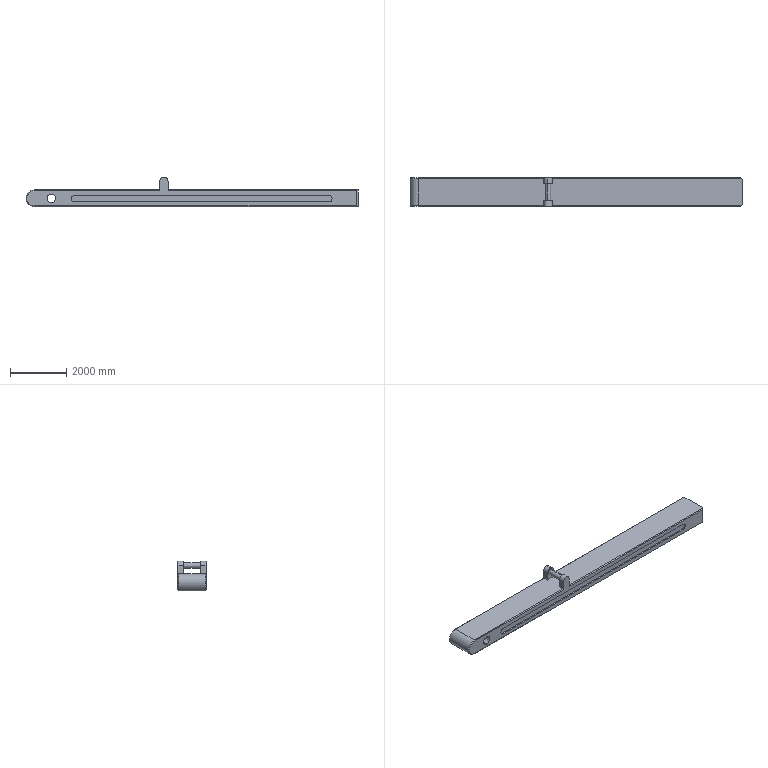Part | SolidWorks | features ICE 4, Chamfer 2, MirrorPattern 2, Extrusion 1 | 1 solid | 44 faces | box 11800 x 1000 x 1050 mm | volume 3596750717 mm3 | plane 30 | cylinder 12 | cone 2 | commonest cylinder face diameters 300 x5 238.236 x4 200 x2 600 x1
STEP:
#1=CARTESIAN_POINT('',(4600.,200.,400.));
#2=VERTEX_POINT('',#1);
#3=CARTESIAN_POINT('',(4600.,200.,200.));
#4=VERTEX_POINT('',#3);
#5=CARTESIAN_POINT('',(4600.,200.,300.));
#6=DIRECTION('',(0.,1.,0.));
#7=DIRECTION('',(0.,0.,-1.));
#8=AXIS2_PLACEMENT_3D('',#5,#6,#7);
#9=CIRCLE('',#8,100.);
#10=EDGE_CURVE('',#2,#4,#9,.T.);
#11=ORIENTED_EDGE('',*,*,#10,.T.);
#12=CARTESIAN_POINT('',(4600.,800.,200.));
#13=VERTEX_POINT('',#12);
#14=CARTESIAN_POINT('',(4600.,100.,200.));
#15=DIRECTION('',(0.,1.,0.));
#16=VECTOR('',#15,1000.);
#17=LINE('',#14,#16);
#18=EDGE_CURVE('',#4,#13,#17,.T.);
#19=ORIENTED_EDGE('',*,*,#18,.T.);
#20=CARTESIAN_POINT('',(4600.,800.,400.));
#21=VERTEX_POINT('',#20);
#22=CARTESIAN_POINT('',(4600.,800.,300.));
#23=DIRECTION('',(0.,-1.,0.));
#24=DIRECTION('',(0.,0.,1.));
#25=AXIS2_PLACEMENT_3D('',#22,#23,#24);
#26=CIRCLE('',#25,100.);
#27=EDGE_CURVE('',#13,#21,#26,.T.);
#28=ORIENTED_EDGE('',*,*,#27,.T.);
#29=CARTESIAN_POINT('',(4600.,100.,400.));
#30=DIRECTION('',(0.,1.,0.));
#31=VECTOR('',#30,1000.);
#32=LINE('',#29,#31);
#33=EDGE_CURVE('',#2,#21,#32,.T.);
#34=ORIENTED_EDGE('',*,*,#33,.F.);
#35=EDGE_LOOP('',(#11,#19,#28,#34));
#36=FACE_OUTER_BOUND('',#35,.T.);
#37=CARTESIAN_POINT('',(4600.,100.,300.));
#38=DIRECTION('',(0.,1.,0.));
#39=DIRECTION('',(0.,0.,1.));
#40=AXIS2_PLACEMENT_3D('',#37,#38,#39);
#41=CYLINDRICAL_SURFACE('',#40,100.);
#42=ADVANCED_FACE('',(#36),#41,.T.);
#43=CARTESIAN_POINT('',(4450.,800.,300.));
#44=VERTEX_POINT('',#43);
#45=CARTESIAN_POINT('',(4600.,800.,450.));
#46=VERTEX_POINT('',#45);
#47=CARTESIAN_POINT('',(4600.,800.,300.));
#48=DIRECTION('',(0.,1.,0.));
#49=DIRECTION('',(0.,0.,1.));
#50=AXIS2_PLACEMENT_3D('',#47,#48,#49);
#51=CIRCLE('',#50,150.);
#52=EDGE_CURVE('',#44,#46,#51,.T.);
#53=ORIENTED_EDGE('',*,*,#52,.T.);
#54=CARTESIAN_POINT('',(4600.,1000.,450.));
#55=VERTEX_POINT('',#54);
#56=CARTESIAN_POINT('',(4600.,800.,450.));
#57=DIRECTION('',(0.,1.,0.));
#58=VECTOR('',#57,1000.);
#59=LINE('',#56,#58);
#60=EDGE_CURVE('',#46,#55,#59,.T.);
#61=ORIENTED_EDGE('',*,*,#60,.T.);
#62=CARTESIAN_POINT('',(4450.,1000.,300.));
#63=VERTEX_POINT('',#62);
#64=CARTESIAN_POINT('',(4600.,1000.,300.));
#65=DIRECTION('',(0.,1.,0.));
#66=DIRECTION('',(0.,0.,1.));
#67=AXIS2_PLACEMENT_3D('',#64,#65,#66);
#68=CIRCLE('',#67,150.);
#69=EDGE_CURVE('',#63,#55,#68,.T.);
#70=ORIENTED_EDGE('',*,*,#69,.F.);
#71=CARTESIAN_POINT('',(4450.,800.,300.));
#72=DIRECTION('',(0.,1.,0.));
#73=VECTOR('',#72,1000.);
#74=LINE('',#71,#73);
#75=EDGE_CURVE('',#44,#63,#74,.T.);
#76=ORIENTED_EDGE('',*,*,#75,.F.);
#77=EDGE_LOOP('',(#53,#61,#70,#76));
#78=FACE_OUTER_BOUND('',#77,.T.);
#79=CARTESIAN_POINT('',(4600.,800.,300.));
#80=DIRECTION('',(0.,1.,0.));
#81=DIRECTION('',(0.,0.,1.));
#82=AXIS2_PLACEMENT_3D('',#79,#80,#81);
#83=CYLINDRICAL_SURFACE('',#82,150.);
#84=ADVANCED_FACE('',(#78),#83,.T.);
#85=CARTESIAN_POINT('',(600.,1000.,-450.));
#86=VERTEX_POINT('',#85);
#87=CARTESIAN_POINT('',(600.,1000.,-150.));
#88=VERTEX_POINT('',#87);
#89=CARTESIAN_POINT('',(600.,1000.,-300.));
#90=DIRECTION('',(0.,1.,0.));
#91=DIRECTION('',(0.,0.,1.));
#92=AXIS2_PLACEMENT_3D('',#89,#90,#91);
#93=CIRCLE('',#92,150.);
#94=EDGE_CURVE('',#86,#88,#93,.T.);
#95=ORIENTED_EDGE('',*,*,#94,.T.);
#96=CARTESIAN_POINT('',(600.,0.,-150.));
#97=VERTEX_POINT('',#96);
#98=CARTESIAN_POINT('',(600.,1000.,-150.));
#99=DIRECTION('',(0.,-1.,0.));
#100=VECTOR('',#99,1000.);
#101=LINE('',#98,#100);
#102=EDGE_CURVE('',#88,#97,#101,.T.);
#103=ORIENTED_EDGE('',*,*,#102,.T.);
#104=CARTESIAN_POINT('',(600.,0.,-450.));
#105=VERTEX_POINT('',#104);
#106=CARTESIAN_POINT('',(600.,0.,-300.));
#107=DIRECTION('',(0.,1.,0.));
#108=DIRECTION('',(0.,0.,1.));
#109=AXIS2_PLACEMENT_3D('',#106,#107,#108);
#110=CIRCLE('',#109,150.);
#111=EDGE_CURVE('',#105,#97,#110,.T.);
#112=ORIENTED_EDGE('',*,*,#111,.F.);
#113=CARTESIAN_POINT('',(600.,1000.,-450.));
#114=DIRECTION('',(0.,-1.,0.));
#115=VECTOR('',#114,1000.);
#116=LINE('',#113,#115);
#117=EDGE_CURVE('',#86,#105,#116,.T.);
#118=ORIENTED_EDGE('',*,*,#117,.F.);
#119=EDGE_LOOP('',(#95,#103,#112,#118));
#120=FACE_OUTER_BOUND('',#119,.T.);
#121=CARTESIAN_POINT('',(600.,1000.,-300.));
#122=DIRECTION('',(0.,-1.,0.));
#123=DIRECTION('',(0.,0.,-1.));
#124=AXIS2_PLACEMENT_3D('',#121,#122,#123);
#125=CYLINDRICAL_SURFACE('',#124,150.);
#126=ADVANCED_FACE('',(#120),#125,.F.);
#127=ORIENTED_EDGE('',*,*,#94,.F.);
#128=CARTESIAN_POINT('',(600.,1000.,-300.));
#129=DIRECTION('',(0.,1.,0.));
#130=DIRECTION('',(0.,0.,1.));
#131=AXIS2_PLACEMENT_3D('',#128,#129,#130);
#132=CIRCLE('',#131,150.);
#133=EDGE_CURVE('',#88,#86,#132,.T.);
#134=ORIENTED_EDGE('',*,*,#133,.F.);
#135=EDGE_LOOP('',(#127,#134));
#136=FACE_BOUND('',#135,.T.);
#137=CARTESIAN_POINT('',(4750.,1000.,-30.));
#138=VERTEX_POINT('',#137);
#139=CARTESIAN_POINT('',(11440.,1000.,-30.));
#140=VERTEX_POINT('',#139);
#141=CARTESIAN_POINT('',(0.,1000.,-30.));
#142=DIRECTION('',(1.,0.,0.));
#143=VECTOR('',#142,1000.);
#144=LINE('',#141,#143);
#145=EDGE_CURVE('',#138,#140,#144,.T.);
#146=ORIENTED_EDGE('',*,*,#145,.T.);
#147=CARTESIAN_POINT('',(11440.,1000.,-570.));
#148=VERTEX_POINT('',#147);
#149=CARTESIAN_POINT('',(11440.,1000.,-300.));
#150=DIRECTION('',(0.,0.,-1.));
#151=VECTOR('',#150,1000.);
#152=LINE('',#149,#151);
#153=EDGE_CURVE('',#140,#148,#152,.T.);
#154=ORIENTED_EDGE('',*,*,#153,.T.);
#155=CARTESIAN_POINT('',(0.,1000.,-570.));
#156=VERTEX_POINT('',#155);
#157=CARTESIAN_POINT('',(0.,1000.,-570.));
#158=DIRECTION('',(-1.,0.,0.));
#159=VECTOR('',#158,1000.);
#160=LINE('',#157,#159);
#161=EDGE_CURVE('',#148,#156,#160,.T.);
#162=ORIENTED_EDGE('',*,*,#161,.T.);
#163=CARTESIAN_POINT('',(0.,1000.,-30.));
#164=VERTEX_POINT('',#163);
#165=CARTESIAN_POINT('',(0.,1000.,-300.));
#166=DIRECTION('',(0.,1.,0.));
#167=DIRECTION('',(0.,0.,-1.));
#168=AXIS2_PLACEMENT_3D('',#165,#166,#167);
#169=CIRCLE('',#168,270.);
#170=EDGE_CURVE('',#156,#164,#169,.T.);
#171=ORIENTED_EDGE('',*,*,#170,.T.);
#172=CARTESIAN_POINT('',(4450.,1000.,-30.));
#173=VERTEX_POINT('',#172);
#174=CARTESIAN_POINT('',(0.,1000.,-30.));
#175=DIRECTION('',(1.,0.,0.));
#176=VECTOR('',#175,1000.);
#177=LINE('',#174,#176);
#178=EDGE_CURVE('',#164,#173,#177,.T.);
#179=ORIENTED_EDGE('',*,*,#178,.T.);
#180=CARTESIAN_POINT('',(4450.,1000.,-203.262));
#181=DIRECTION('',(0.,0.,1.));
#182=VECTOR('',#181,1000.);
#183=LINE('',#180,#182);
#184=EDGE_CURVE('',#173,#63,#183,.T.);
#185=ORIENTED_EDGE('',*,*,#184,.T.);
#186=ORIENTED_EDGE('',*,*,#69,.T.);
#187=CARTESIAN_POINT('',(4750.,1000.,300.));
#188=VERTEX_POINT('',#187);
#189=CARTESIAN_POINT('',(4600.,1000.,300.));
#190=DIRECTION('',(0.,1.,0.));
#191=DIRECTION('',(0.,0.,1.));
#192=AXIS2_PLACEMENT_3D('',#189,#190,#191);
#193=CIRCLE('',#192,150.);
#194=EDGE_CURVE('',#55,#188,#193,.T.);
#195=ORIENTED_EDGE('',*,*,#194,.T.);
#196=CARTESIAN_POINT('',(4750.,1000.,-203.262));
#197=DIRECTION('',(0.,0.,-1.));
#198=VECTOR('',#197,1000.);
#199=LINE('',#196,#198);
#200=EDGE_CURVE('',#188,#138,#199,.T.);
#201=ORIENTED_EDGE('',*,*,#200,.T.);
#202=EDGE_LOOP('',(#146,#154,#162,#171,#179,#185,#186,#195,#201));
#203=FACE_OUTER_BOUND('',#202,.T.);
#204=CARTESIAN_POINT('',(1432.066,1000.,-188.683));
#205=VERTEX_POINT('',#204);
#206=CARTESIAN_POINT('',(1432.066,1000.,-426.919));
#207=VERTEX_POINT('',#206);
#208=CARTESIAN_POINT('',(1432.066,1000.,-307.801));
#209=DIRECTION('',(0.,-1.,0.));
#210=DIRECTION('',(0.,0.,-1.));
#211=AXIS2_PLACEMENT_3D('',#208,#209,#210);
#212=CIRCLE('',#211,119.118);
#213=EDGE_CURVE('',#205,#207,#212,.T.);
#214=ORIENTED_EDGE('',*,*,#213,.T.);
#215=CARTESIAN_POINT('',(10462.796,1000.,-426.919));
#216=VERTEX_POINT('',#215);
#217=CARTESIAN_POINT('',(1432.066,1000.,-426.919));
#218=DIRECTION('',(1.,0.,0.));
#219=VECTOR('',#218,1000.);
#220=LINE('',#217,#219);
#221=EDGE_CURVE('',#207,#216,#220,.T.);
#222=ORIENTED_EDGE('',*,*,#221,.T.);
#223=CARTESIAN_POINT('',(10462.796,1000.,-188.683));
#224=VERTEX_POINT('',#223);
#225=CARTESIAN_POINT('',(10462.796,1000.,-307.801));
#226=DIRECTION('',(0.,-1.,0.));
#227=DIRECTION('',(0.,0.,-1.));
#228=AXIS2_PLACEMENT_3D('',#225,#226,#227);
#229=CIRCLE('',#228,119.118);
#230=EDGE_CURVE('',#216,#224,#229,.T.);
#231=ORIENTED_EDGE('',*,*,#230,.T.);
#232=CARTESIAN_POINT('',(1432.066,1000.,-188.683));
#233=DIRECTION('',(-1.,0.,0.));
#234=VECTOR('',#233,1000.);
#235=LINE('',#232,#234);
#236=EDGE_CURVE('',#224,#205,#235,.T.);
#237=ORIENTED_EDGE('',*,*,#236,.T.);
#238=EDGE_LOOP('',(#214,#222,#231,#237));
#239=FACE_BOUND('',#238,.T.);
#240=CARTESIAN_POINT('',(0.,1000.,-300.));
#241=DIRECTION('',(0.,-1.,0.));
#242=DIRECTION('',(0.,0.,-1.));
#243=AXIS2_PLACEMENT_3D('',#240,#241,#242);
#244=PLANE('',#243);
#245=ADVANCED_FACE('',(#136,#203,#239),#244,.F.);
#246=CARTESIAN_POINT('',(11500.,940.,0.));
#247=VERTEX_POINT('',#246);
#248=CARTESIAN_POINT('',(11500.,60.,0.));
#249=VERTEX_POINT('',#248);
#250=CARTESIAN_POINT('',(11500.,1000.,0.));
#251=DIRECTION('',(0.,-1.,0.));
#252=VECTOR('',#251,1000.);
#253=LINE('',#250,#252);
#254=EDGE_CURVE('',#247,#249,#253,.T.);
#255=ORIENTED_EDGE('',*,*,#254,.F.);
#256=CARTESIAN_POINT('',(11470.,970.,0.));
#257=VERTEX_POINT('',#256);
#258=CARTESIAN_POINT('',(11440.,1000.,0.));
#259=DIRECTION('',(-0.7071,0.7071,0.));
#260=VECTOR('',#259,1000.);
#261=LINE('',#258,#260);
#262=EDGE_CURVE('',#247,#257,#261,.T.);
#263=ORIENTED_EDGE('',*,*,#262,.T.);
#264=CARTESIAN_POINT('',(4750.,970.,0.));
#265=VERTEX_POINT('',#264);
#266=CARTESIAN_POINT('',(0.,970.,0.));
#267=DIRECTION('',(-1.,0.,0.));
#268=VECTOR('',#267,1000.);
#269=LINE('',#266,#268);
#270=EDGE_CURVE('',#257,#265,#269,.T.);
#271=ORIENTED_EDGE('',*,*,#270,.T.);
#272=CARTESIAN_POINT('',(4750.,800.,0.));
#273=VERTEX_POINT('',#272);
#274=CARTESIAN_POINT('',(4750.,1000.,0.));
#275=DIRECTION('',(0.,-1.,0.));
#276=VECTOR('',#275,1000.);
#277=LINE('',#274,#276);
#278=EDGE_CURVE('',#265,#273,#277,.T.);
#279=ORIENTED_EDGE('',*,*,#278,.T.);
#280=CARTESIAN_POINT('',(4450.,800.,0.));
#281=VERTEX_POINT('',#280);
#282=CARTESIAN_POINT('',(0.,800.,0.));
#283=DIRECTION('',(1.,0.,0.));
#284=VECTOR('',#283,1000.);
#285=LINE('',#282,#284);
#286=EDGE_CURVE('',#281,#273,#285,.T.);
#287=ORIENTED_EDGE('',*,*,#286,.F.);
#288=CARTESIAN_POINT('',(4450.,970.,0.));
#289=VERTEX_POINT('',#288);
#290=CARTESIAN_POINT('',(4450.,1000.,0.));
#291=DIRECTION('',(0.,1.,0.));
#292=VECTOR('',#291,1000.);
#293=LINE('',#290,#292);
#294=EDGE_CURVE('',#281,#289,#293,.T.);
#295=ORIENTED_EDGE('',*,*,#294,.T.);
#296=CARTESIAN_POINT('',(0.,970.,0.));
#297=VERTEX_POINT('',#296);
#298=CARTESIAN_POINT('',(0.,970.,0.));
#299=DIRECTION('',(-1.,0.,0.));
#300=VECTOR('',#299,1000.);
#301=LINE('',#298,#300);
#302=EDGE_CURVE('',#289,#297,#301,.T.);
#303=ORIENTED_EDGE('',*,*,#302,.T.);
#304=CARTESIAN_POINT('',(0.,30.,0.));
#305=VERTEX_POINT('',#304);
#306=CARTESIAN_POINT('',(0.,1000.,0.));
#307=DIRECTION('',(0.,-1.,0.));
#308=VECTOR('',#307,1000.);
#309=LINE('',#306,#308);
#310=EDGE_CURVE('',#297,#305,#309,.T.);
#311=ORIENTED_EDGE('',*,*,#310,.T.);
#312=CARTESIAN_POINT('',(4450.,30.,0.));
#313=VERTEX_POINT('',#312);
#314=CARTESIAN_POINT('',(4450.,30.,0.));
#315=DIRECTION('',(1.,0.,0.));
#316=VECTOR('',#315,1000.);
#317=LINE('',#314,#316);
#318=EDGE_CURVE('',#305,#313,#317,.T.);
#319=ORIENTED_EDGE('',*,*,#318,.T.);
#320=CARTESIAN_POINT('',(4450.,200.,0.));
#321=VERTEX_POINT('',#320);
#322=CARTESIAN_POINT('',(4450.,1000.,0.));
#323=DIRECTION('',(0.,-1.,0.));
#324=VECTOR('',#323,1000.);
#325=LINE('',#322,#324);
#326=EDGE_CURVE('',#321,#313,#325,.T.);
#327=ORIENTED_EDGE('',*,*,#326,.F.);
#328=CARTESIAN_POINT('',(4750.,200.,0.));
#329=VERTEX_POINT('',#328);
#330=CARTESIAN_POINT('',(0.,200.,0.));
#331=DIRECTION('',(-1.,0.,0.));
#332=VECTOR('',#331,1000.);
#333=LINE('',#330,#332);
#334=EDGE_CURVE('',#329,#321,#333,.T.);
#335=ORIENTED_EDGE('',*,*,#334,.F.);
#336=CARTESIAN_POINT('',(4750.,30.,0.));
#337=VERTEX_POINT('',#336);
#338=CARTESIAN_POINT('',(4750.,1000.,0.));
#339=DIRECTION('',(0.,1.,0.));
#340=VECTOR('',#339,1000.);
#341=LINE('',#338,#340);
#342=EDGE_CURVE('',#337,#329,#341,.T.);
#343=ORIENTED_EDGE('',*,*,#342,.F.);
#344=CARTESIAN_POINT('',(11470.,30.,0.));
#345=VERTEX_POINT('',#344);
#346=CARTESIAN_POINT('',(11500.,30.,0.));
#347=DIRECTION('',(1.,0.,0.));
#348=VECTOR('',#347,1000.);
#349=LINE('',#346,#348);
#350=EDGE_CURVE('',#337,#345,#349,.T.);
#351=ORIENTED_EDGE('',*,*,#350,.T.);
#352=CARTESIAN_POINT('',(11500.,60.,0.));
#353=DIRECTION('',(0.7071,0.7071,0.));
#354=VECTOR('',#353,1000.);
#355=LINE('',#352,#354);
#356=EDGE_CURVE('',#345,#249,#355,.T.);
#357=ORIENTED_EDGE('',*,*,#356,.T.);
#358=EDGE_LOOP('',(#255,#263,#271,#279,#287,#295,#303,#311,#319,#327,#335,#343,#351,#357));
#359=FACE_OUTER_BOUND('',#358,.T.);
#360=CARTESIAN_POINT('',(0.,1000.,0.));
#361=DIRECTION('',(0.,0.,-1.));
#362=DIRECTION('',(-1.,0.,0.));
#363=AXIS2_PLACEMENT_3D('',#360,#361,#362);
#364=PLANE('',#363);
#365=ADVANCED_FACE('',(#359),#364,.F.);
#366=CARTESIAN_POINT('',(1432.066,0.,-188.683));
#367=VERTEX_POINT('',#366);
#368=CARTESIAN_POINT('',(1432.066,0.,-426.919));
#369=VERTEX_POINT('',#368);
#370=CARTESIAN_POINT('',(1432.066,0.,-307.801));
#371=DIRECTION('',(0.,-1.,0.));
#372=DIRECTION('',(0.,0.,-1.));
#373=AXIS2_PLACEMENT_3D('',#370,#371,#372);
#374=CIRCLE('',#373,119.118);
#375=EDGE_CURVE('',#367,#369,#374,.T.);
#376=ORIENTED_EDGE('',*,*,#375,.F.);
#377=CARTESIAN_POINT('',(10462.796,0.,-188.683));
#378=VERTEX_POINT('',#377);
#379=CARTESIAN_POINT('',(1432.066,0.,-188.683));
#380=DIRECTION('',(-1.,0.,0.));
#381=VECTOR('',#380,1000.);
#382=LINE('',#379,#381);
#383=EDGE_CURVE('',#378,#367,#382,.T.);
#384=ORIENTED_EDGE('',*,*,#383,.F.);
#385=CARTESIAN_POINT('',(10462.796,0.,-426.919));
#386=VERTEX_POINT('',#385);
#387=CARTESIAN_POINT('',(10462.796,0.,-307.801));
#388=DIRECTION('',(0.,-1.,0.));
#389=DIRECTION('',(0.,0.,-1.));
#390=AXIS2_PLACEMENT_3D('',#387,#388,#389);
#391=CIRCLE('',#390,119.118);
#392=EDGE_CURVE('',#386,#378,#391,.T.);
#393=ORIENTED_EDGE('',*,*,#392,.F.);
#394=CARTESIAN_POINT('',(1432.066,0.,-426.919));
#395=DIRECTION('',(1.,0.,0.));
#396=VECTOR('',#395,1000.);
#397=LINE('',#394,#396);
#398=EDGE_CURVE('',#369,#386,#397,.T.);
#399=ORIENTED_EDGE('',*,*,#398,.F.);
#400=EDGE_LOOP('',(#376,#384,#393,#399));
#401=FACE_BOUND('',#400,.T.);
#402=CARTESIAN_POINT('',(0.,0.,-570.));
#403=VERTEX_POINT('',#402);
#404=CARTESIAN_POINT('',(11440.,0.,-570.));
#405=VERTEX_POINT('',#404);
#406=CARTESIAN_POINT('',(11500.,0.,-570.));
#407=DIRECTION('',(1.,0.,0.));
#408=VECTOR('',#407,1000.);
#409=LINE('',#406,#408);
#410=EDGE_CURVE('',#403,#405,#409,.T.);
#411=ORIENTED_EDGE('',*,*,#410,.T.);
#412=CARTESIAN_POINT('',(11440.,0.,-30.));
#413=VERTEX_POINT('',#412);
#414=CARTESIAN_POINT('',(11440.,0.,-30.));
#415=DIRECTION('',(0.,0.,1.));
#416=VECTOR('',#415,1000.);
#417=LINE('',#414,#416);
#418=EDGE_CURVE('',#405,#413,#417,.T.);
#419=ORIENTED_EDGE('',*,*,#418,.T.);
#420=CARTESIAN_POINT('',(4750.,0.,-30.));
#421=VERTEX_POINT('',#420);
#422=CARTESIAN_POINT('',(4750.,0.,-30.));
#423=DIRECTION('',(-1.,0.,0.));
#424=VECTOR('',#423,1000.);
#425=LINE('',#422,#424);
#426=EDGE_CURVE('',#413,#421,#425,.T.);
#427=ORIENTED_EDGE('',*,*,#426,.T.);
#428=CARTESIAN_POINT('',(4750.,0.,300.));
#429=VERTEX_POINT('',#428);
#430=CARTESIAN_POINT('',(4750.,0.,-203.262));
#431=DIRECTION('',(0.,0.,-1.));
#432=VECTOR('',#431,1000.);
#433=LINE('',#430,#432);
#434=EDGE_CURVE('',#429,#421,#433,.T.);
#435=ORIENTED_EDGE('',*,*,#434,.F.);
#436=CARTESIAN_POINT('',(4450.,0.,300.));
#437=VERTEX_POINT('',#436);
#438=CARTESIAN_POINT('',(4600.,0.,300.));
#439=DIRECTION('',(0.,1.,0.));
#440=DIRECTION('',(0.,0.,1.));
#441=AXIS2_PLACEMENT_3D('',#438,#439,#440);
#442=CIRCLE('',#441,150.);
#443=EDGE_CURVE('',#437,#429,#442,.T.);
#444=ORIENTED_EDGE('',*,*,#443,.F.);
#445=CARTESIAN_POINT('',(4450.,0.,-30.));
#446=VERTEX_POINT('',#445);
#447=CARTESIAN_POINT('',(4450.,0.,-203.262));
#448=DIRECTION('',(0.,0.,1.));
#449=VECTOR('',#448,1000.);
#450=LINE('',#447,#449);
#451=EDGE_CURVE('',#446,#437,#450,.T.);
#452=ORIENTED_EDGE('',*,*,#451,.F.);
#453=CARTESIAN_POINT('',(0.,0.,-30.));
#454=VERTEX_POINT('',#453);
#455=CARTESIAN_POINT('',(0.,0.,-30.));
#456=DIRECTION('',(-1.,0.,0.));
#457=VECTOR('',#456,1000.);
#458=LINE('',#455,#457);
#459=EDGE_CURVE('',#446,#454,#458,.T.);
#460=ORIENTED_EDGE('',*,*,#459,.T.);
#461=CARTESIAN_POINT('',(0.,0.,-300.));
#462=DIRECTION('',(0.,-1.,0.));
#463=DIRECTION('',(0.,0.,-1.));
#464=AXIS2_PLACEMENT_3D('',#461,#462,#463);
#465=CIRCLE('',#464,270.);
#466=EDGE_CURVE('',#454,#403,#465,.T.);
#467=ORIENTED_EDGE('',*,*,#466,.T.);
#468=EDGE_LOOP('',(#411,#419,#427,#435,#444,#452,#460,#467));
#469=FACE_OUTER_BOUND('',#468,.T.);
#470=ORIENTED_EDGE('',*,*,#111,.T.);
#471=CARTESIAN_POINT('',(600.,0.,-300.));
#472=DIRECTION('',(0.,1.,0.));
#473=DIRECTION('',(0.,0.,1.));
#474=AXIS2_PLACEMENT_3D('',#471,#472,#473);
#475=CIRCLE('',#474,150.);
#476=EDGE_CURVE('',#97,#105,#475,.T.);
#477=ORIENTED_EDGE('',*,*,#476,.T.);
#478=EDGE_LOOP('',(#470,#477));
#479=FACE_BOUND('',#478,.T.);
#480=CARTESIAN_POINT('',(0.,0.,-300.));
#481=DIRECTION('',(0.,-1.,0.));
#482=DIRECTION('',(0.,0.,-1.));
#483=AXIS2_PLACEMENT_3D('',#480,#481,#482);
#484=PLANE('',#483);
#485=ADVANCED_FACE('',(#401,#469,#479),#484,.T.);
#486=ORIENTED_EDGE('',*,*,#310,.F.);
#487=CARTESIAN_POINT('',(0.,970.,-600.));
#488=VERTEX_POINT('',#487);
#489=CARTESIAN_POINT('',(0.,970.,-300.));
#490=DIRECTION('',(0.,-1.,0.));
#491=DIRECTION('',(0.,0.,-1.));
#492=AXIS2_PLACEMENT_3D('',#489,#490,#491);
#493=CIRCLE('',#492,300.);
#494=EDGE_CURVE('',#297,#488,#493,.T.);
#495=ORIENTED_EDGE('',*,*,#494,.T.);
#496=CARTESIAN_POINT('',(0.,30.,-600.));
#497=VERTEX_POINT('',#496);
#498=CARTESIAN_POINT('',(0.,1000.,-600.));
#499=DIRECTION('',(0.,-1.,0.));
#500=VECTOR('',#499,1000.);
#501=LINE('',#498,#500);
#502=EDGE_CURVE('',#488,#497,#501,.T.);
#503=ORIENTED_EDGE('',*,*,#502,.T.);
#504=CARTESIAN_POINT('',(0.,30.,-300.));
#505=DIRECTION('',(0.,1.,0.));
#506=DIRECTION('',(0.,0.,-1.));
#507=AXIS2_PLACEMENT_3D('',#504,#505,#506);
#508=CIRCLE('',#507,300.);
#509=EDGE_CURVE('',#497,#305,#508,.T.);
#510=ORIENTED_EDGE('',*,*,#509,.T.);
#511=EDGE_LOOP('',(#486,#495,#503,#510));
#512=FACE_OUTER_BOUND('',#511,.T.);
#513=CARTESIAN_POINT('',(0.,1000.,-300.));
#514=DIRECTION('',(0.,-1.,0.));
#515=DIRECTION('',(0.,0.,-1.));
#516=AXIS2_PLACEMENT_3D('',#513,#514,#515);
#517=CYLINDRICAL_SURFACE('',#516,300.);
#518=ADVANCED_FACE('',(#512),#517,.T.);
#519=CARTESIAN_POINT('',(11500.,100.,-100.));
#520=VERTEX_POINT('',#519);
#521=CARTESIAN_POINT('',(11500.,100.,-500.));
#522=VERTEX_POINT('',#521);
#523=CARTESIAN_POINT('',(11500.,100.,-100.));
#524=DIRECTION('',(0.,0.,-1.));
#525=VECTOR('',#524,1000.);
#526=LINE('',#523,#525);
#527=EDGE_CURVE('',#520,#522,#526,.T.);
#528=ORIENTED_EDGE('',*,*,#527,.F.);
#529=CARTESIAN_POINT('',(11500.,900.,-100.));
#530=VERTEX_POINT('',#529);
#531=CARTESIAN_POINT('',(11500.,900.,-100.));
#532=DIRECTION('',(0.,-1.,0.));
#533=VECTOR('',#532,1000.);
#534=LINE('',#531,#533);
#535=EDGE_CURVE('',#530,#520,#534,.T.);
#536=ORIENTED_EDGE('',*,*,#535,.F.);
#537=CARTESIAN_POINT('',(11500.,900.,-500.));
#538=VERTEX_POINT('',#537);
#539=CARTESIAN_POINT('',(11500.,900.,-100.));
#540=DIRECTION('',(0.,0.,1.));
#541=VECTOR('',#540,1000.);
#542=LINE('',#539,#541);
#543=EDGE_CURVE('',#538,#530,#542,.T.);
#544=ORIENTED_EDGE('',*,*,#543,.F.);
#545=CARTESIAN_POINT('',(11500.,900.,-500.));
#546=DIRECTION('',(0.,1.,0.));
#547=VECTOR('',#546,1000.);
#548=LINE('',#545,#547);
#549=EDGE_CURVE('',#522,#538,#548,.T.);
#550=ORIENTED_EDGE('',*,*,#549,.F.);
#551=EDGE_LOOP('',(#528,#536,#544,#550));
#552=FACE_BOUND('',#551,.T.);
#553=CARTESIAN_POINT('',(11500.,940.,-600.));
#554=VERTEX_POINT('',#553);
#555=CARTESIAN_POINT('',(11500.,60.,-600.));
#556=VERTEX_POINT('',#555);
#557=CARTESIAN_POINT('',(11500.,1000.,-600.));
#558=DIRECTION('',(0.,-1.,0.));
#559=VECTOR('',#558,1000.);
#560=LINE('',#557,#559);
#561=EDGE_CURVE('',#554,#556,#560,.T.);
#562=ORIENTED_EDGE('',*,*,#561,.F.);
#563=CARTESIAN_POINT('',(11500.,940.,0.));
#564=DIRECTION('',(0.,0.,1.));
#565=VECTOR('',#564,1000.);
#566=LINE('',#563,#565);
#567=EDGE_CURVE('',#554,#247,#566,.T.);
#568=ORIENTED_EDGE('',*,*,#567,.T.);
#569=ORIENTED_EDGE('',*,*,#254,.T.);
#570=CARTESIAN_POINT('',(11500.,60.,-570.));
#571=DIRECTION('',(0.,0.,-1.));
#572=VECTOR('',#571,1000.);
#573=LINE('',#570,#572);
#574=EDGE_CURVE('',#249,#556,#573,.T.);
#575=ORIENTED_EDGE('',*,*,#574,.T.);
#576=EDGE_LOOP('',(#562,#568,#569,#575));
#577=FACE_OUTER_BOUND('',#576,.T.);
#578=CARTESIAN_POINT('',(11500.,1000.,0.));
#579=DIRECTION('',(-1.,0.,0.));
#580=DIRECTION('',(0.,0.,1.));
#581=AXIS2_PLACEMENT_3D('',#578,#579,#580);
#582=PLANE('',#581);
#583=ADVANCED_FACE('',(#552,#577),#582,.F.);
#584=CARTESIAN_POINT('',(11470.,970.,-600.));
#585=VERTEX_POINT('',#584);
#586=CARTESIAN_POINT('',(0.,970.,-600.));
#587=DIRECTION('',(1.,0.,0.));
#588=VECTOR('',#587,1000.);
#589=LINE('',#586,#588);
#590=EDGE_CURVE('',#488,#585,#589,.T.);
#591=ORIENTED_EDGE('',*,*,#590,.T.);
#592=CARTESIAN_POINT('',(11440.,1000.,-600.));
#593=DIRECTION('',(0.7071,-0.7071,0.));
#594=VECTOR('',#593,1000.);
#595=LINE('',#592,#594);
#596=EDGE_CURVE('',#585,#554,#595,.T.);
#597=ORIENTED_EDGE('',*,*,#596,.T.);
#598=ORIENTED_EDGE('',*,*,#561,.T.);
#599=CARTESIAN_POINT('',(11470.,30.,-600.));
#600=VERTEX_POINT('',#599);
#601=CARTESIAN_POINT('',(11500.,60.,-600.));
#602=DIRECTION('',(-0.7071,-0.7071,0.));
#603=VECTOR('',#602,1000.);
#604=LINE('',#601,#603);
#605=EDGE_CURVE('',#556,#600,#604,.T.);
#606=ORIENTED_EDGE('',*,*,#605,.T.);
#607=CARTESIAN_POINT('',(0.,30.,-600.));
#608=DIRECTION('',(-1.,0.,0.));
#609=VECTOR('',#608,1000.);
#610=LINE('',#607,#609);
#611=EDGE_CURVE('',#600,#497,#610,.T.);
#612=ORIENTED_EDGE('',*,*,#611,.T.);
#613=ORIENTED_EDGE('',*,*,#502,.F.);
#614=EDGE_LOOP('',(#591,#597,#598,#606,#612,#613));
#615=FACE_OUTER_BOUND('',#614,.T.);
#616=CARTESIAN_POINT('',(0.,1000.,-600.));
#617=DIRECTION('',(0.,0.,1.));
#618=DIRECTION('',(1.,0.,0.));
#619=AXIS2_PLACEMENT_3D('',#616,#617,#618);
#620=PLANE('',#619);
#621=ADVANCED_FACE('',(#615),#620,.F.);
#622=ORIENTED_EDGE('',*,*,#102,.F.);
#623=ORIENTED_EDGE('',*,*,#133,.T.);
#624=ORIENTED_EDGE('',*,*,#117,.T.);
#625=ORIENTED_EDGE('',*,*,#476,.F.);
#626=EDGE_LOOP('',(#622,#623,#624,#625));
#627=FACE_OUTER_BOUND('',#626,.T.);
#628=CARTESIAN_POINT('',(600.,1000.,-300.));
#629=DIRECTION('',(0.,-1.,0.));
#630=DIRECTION('',(0.,0.,-1.));
#631=AXIS2_PLACEMENT_3D('',#628,#629,#630);
#632=CYLINDRICAL_SURFACE('',#631,150.);
#633=ADVANCED_FACE('',(#627),#632,.F.);
#634=ORIENTED_EDGE('',*,*,#278,.F.);
#635=CARTESIAN_POINT('',(4750.,1000.,-30.));
#636=DIRECTION('',(0.,0.7071,-0.7071));
#637=VECTOR('',#636,1000.);
#638=LINE('',#635,#637);
#639=EDGE_CURVE('',#265,#138,#638,.T.);
#640=ORIENTED_EDGE('',*,*,#639,.T.);
#641=ORIENTED_EDGE('',*,*,#200,.F.);
#642=CARTESIAN_POINT('',(4750.,800.,300.));
#643=VERTEX_POINT('',#642);
#644=CARTESIAN_POINT('',(4750.,800.,300.));
#645=DIRECTION('',(0.,1.,0.));
#646=VECTOR('',#645,1000.);
#647=LINE('',#644,#646);
#648=EDGE_CURVE('',#643,#188,#647,.T.);
#649=ORIENTED_EDGE('',*,*,#648,.F.);
#650=CARTESIAN_POINT('',(4750.,800.,-203.262));
#651=DIRECTION('',(0.,0.,-1.));
#652=VECTOR('',#651,1000.);
#653=LINE('',#650,#652);
#654=EDGE_CURVE('',#643,#273,#653,.T.);
#655=ORIENTED_EDGE('',*,*,#654,.T.);
#656=EDGE_LOOP('',(#634,#640,#641,#649,#655));
#657=FACE_OUTER_BOUND('',#656,.T.);
#658=CARTESIAN_POINT('',(4750.,800.,-203.262));
#659=DIRECTION('',(1.,0.,0.));
#660=DIRECTION('',(0.,0.,-1.));
#661=AXIS2_PLACEMENT_3D('',#658,#659,#660);
#662=PLANE('',#661);
#663=ADVANCED_FACE('',(#657),#662,.T.);
#664=ORIENTED_EDGE('',*,*,#294,.F.);
#665=CARTESIAN_POINT('',(4450.,800.,-203.262));
#666=DIRECTION('',(0.,0.,1.));
#667=VECTOR('',#666,1000.);
#668=LINE('',#665,#667);
#669=EDGE_CURVE('',#281,#44,#668,.T.);
#670=ORIENTED_EDGE('',*,*,#669,.T.);
#671=ORIENTED_EDGE('',*,*,#75,.T.);
#672=ORIENTED_EDGE('',*,*,#184,.F.);
#673=CARTESIAN_POINT('',(4450.,1000.,-30.));
#674=DIRECTION('',(0.,-0.7071,0.7071));
#675=VECTOR('',#674,1000.);
#676=LINE('',#673,#675);
#677=EDGE_CURVE('',#173,#289,#676,.T.);
#678=ORIENTED_EDGE('',*,*,#677,.T.);
#679=EDGE_LOOP('',(#664,#670,#671,#672,#678));
#680=FACE_OUTER_BOUND('',#679,.T.);
#681=CARTESIAN_POINT('',(4450.,800.,-203.262));
#682=DIRECTION('',(-1.,0.,0.));
#683=DIRECTION('',(0.,0.,1.));
#684=AXIS2_PLACEMENT_3D('',#681,#682,#683);
#685=PLANE('',#684);
#686=ADVANCED_FACE('',(#680),#685,.T.);
#687=CARTESIAN_POINT('',(4600.,800.,300.));
#688=DIRECTION('',(0.,-1.,0.));
#689=DIRECTION('',(0.,0.,1.));
#690=AXIS2_PLACEMENT_3D('',#687,#688,#689);
#691=CIRCLE('',#690,100.);
#692=EDGE_CURVE('',#21,#13,#691,.T.);
#693=ORIENTED_EDGE('',*,*,#692,.F.);
#694=ORIENTED_EDGE('',*,*,#27,.F.);
#695=EDGE_LOOP('',(#693,#694));
#696=FACE_BOUND('',#695,.T.);
#697=ORIENTED_EDGE('',*,*,#669,.F.);
#698=ORIENTED_EDGE('',*,*,#286,.T.);
#699=ORIENTED_EDGE('',*,*,#654,.F.);
#700=CARTESIAN_POINT('',(4600.,800.,300.));
#701=DIRECTION('',(0.,1.,0.));
#702=DIRECTION('',(0.,0.,1.));
#703=AXIS2_PLACEMENT_3D('',#700,#701,#702);
#704=CIRCLE('',#703,150.);
#705=EDGE_CURVE('',#46,#643,#704,.T.);
#706=ORIENTED_EDGE('',*,*,#705,.F.);
#707=ORIENTED_EDGE('',*,*,#52,.F.);
#708=EDGE_LOOP('',(#697,#698,#699,#706,#707));
#709=FACE_OUTER_BOUND('',#708,.T.);
#710=CARTESIAN_POINT('',(4600.,800.,-203.262));
#711=DIRECTION('',(0.,1.,0.));
#712=DIRECTION('',(0.,0.,1.));
#713=AXIS2_PLACEMENT_3D('',#710,#711,#712);
#714=PLANE('',#713);
#715=ADVANCED_FACE('',(#696,#709),#714,.F.);
#716=ORIENTED_EDGE('',*,*,#60,.F.);
#717=ORIENTED_EDGE('',*,*,#705,.T.);
#718=ORIENTED_EDGE('',*,*,#648,.T.);
#719=ORIENTED_EDGE('',*,*,#194,.F.);
#720=EDGE_LOOP('',(#716,#717,#718,#719));
#721=FACE_OUTER_BOUND('',#720,.T.);
#722=CARTESIAN_POINT('',(4600.,800.,300.));
#723=DIRECTION('',(0.,1.,0.));
#724=DIRECTION('',(0.,0.,1.));
#725=AXIS2_PLACEMENT_3D('',#722,#723,#724);
#726=CYLINDRICAL_SURFACE('',#725,150.);
#727=ADVANCED_FACE('',(#721),#726,.T.);
#728=CARTESIAN_POINT('',(4450.,200.,300.));
#729=VERTEX_POINT('',#728);
#730=CARTESIAN_POINT('',(4450.,200.,-203.262));
#731=DIRECTION('',(0.,0.,1.));
#732=VECTOR('',#731,1000.);
#733=LINE('',#730,#732);
#734=EDGE_CURVE('',#321,#729,#733,.T.);
#735=ORIENTED_EDGE('',*,*,#734,.F.);
#736=ORIENTED_EDGE('',*,*,#326,.T.);
#737=CARTESIAN_POINT('',(4450.,13.369,-16.631));
#738=DIRECTION('',(0.,-0.7071,-0.7071));
#739=VECTOR('',#738,1000.);
#740=LINE('',#737,#739);
#741=EDGE_CURVE('',#313,#446,#740,.T.);
#742=ORIENTED_EDGE('',*,*,#741,.T.);
#743=ORIENTED_EDGE('',*,*,#451,.T.);
#744=CARTESIAN_POINT('',(4450.,200.,300.));
#745=DIRECTION('',(0.,-1.,0.));
#746=VECTOR('',#745,1000.);
#747=LINE('',#744,#746);
#748=EDGE_CURVE('',#729,#437,#747,.T.);
#749=ORIENTED_EDGE('',*,*,#748,.F.);
#750=EDGE_LOOP('',(#735,#736,#742,#743,#749));
#751=FACE_OUTER_BOUND('',#750,.T.);
#752=CARTESIAN_POINT('',(4450.,200.,-203.262));
#753=DIRECTION('',(1.,0.,0.));
#754=DIRECTION('',(0.,0.,-1.));
#755=AXIS2_PLACEMENT_3D('',#752,#753,#754);
#756=PLANE('',#755);
#757=ADVANCED_FACE('',(#751),#756,.F.);
#758=ORIENTED_EDGE('',*,*,#434,.T.);
#759=CARTESIAN_POINT('',(4750.,13.369,-16.631));
#760=DIRECTION('',(0.,0.7071,0.7071));
#761=VECTOR('',#760,1000.);
#762=LINE('',#759,#761);
#763=EDGE_CURVE('',#421,#337,#762,.T.);
#764=ORIENTED_EDGE('',*,*,#763,.T.);
#765=ORIENTED_EDGE('',*,*,#342,.T.);
#766=CARTESIAN_POINT('',(4750.,200.,300.));
#767=VERTEX_POINT('',#766);
#768=CARTESIAN_POINT('',(4750.,200.,-203.262));
#769=DIRECTION('',(0.,0.,-1.));
#770=VECTOR('',#769,1000.);
#771=LINE('',#768,#770);
#772=EDGE_CURVE('',#767,#329,#771,.T.);
#773=ORIENTED_EDGE('',*,*,#772,.F.);
#774=CARTESIAN_POINT('',(4750.,200.,300.));
#775=DIRECTION('',(0.,-1.,0.));
#776=VECTOR('',#775,1000.);
#777=LINE('',#774,#776);
#778=EDGE_CURVE('',#767,#429,#777,.T.);
#779=ORIENTED_EDGE('',*,*,#778,.T.);
#780=EDGE_LOOP('',(#758,#764,#765,#773,#779));
#781=FACE_OUTER_BOUND('',#780,.T.);
#782=CARTESIAN_POINT('',(4750.,200.,-203.262));
#783=DIRECTION('',(-1.,0.,0.));
#784=DIRECTION('',(0.,0.,1.));
#785=AXIS2_PLACEMENT_3D('',#782,#783,#784);
#786=PLANE('',#785);
#787=ADVANCED_FACE('',(#781),#786,.F.);
#788=ORIENTED_EDGE('',*,*,#10,.F.);
#789=CARTESIAN_POINT('',(4600.,200.,300.));
#790=DIRECTION('',(0.,1.,0.));
#791=DIRECTION('',(0.,0.,-1.));
#792=AXIS2_PLACEMENT_3D('',#789,#790,#791);
#793=CIRCLE('',#792,100.);
#794=EDGE_CURVE('',#4,#2,#793,.T.);
#795=ORIENTED_EDGE('',*,*,#794,.F.);
#796=EDGE_LOOP('',(#788,#795));
#797=FACE_BOUND('',#796,.T.);
#798=ORIENTED_EDGE('',*,*,#772,.T.);
#799=ORIENTED_EDGE('',*,*,#334,.T.);
#800=ORIENTED_EDGE('',*,*,#734,.T.);
#801=CARTESIAN_POINT('',(4600.,200.,300.));
#802=DIRECTION('',(0.,1.,0.));
#803=DIRECTION('',(0.,0.,1.));
#804=AXIS2_PLACEMENT_3D('',#801,#802,#803);
#805=CIRCLE('',#804,150.);
#806=EDGE_CURVE('',#729,#767,#805,.T.);
#807=ORIENTED_EDGE('',*,*,#806,.T.);
#808=EDGE_LOOP('',(#798,#799,#800,#807));
#809=FACE_OUTER_BOUND('',#808,.T.);
#810=CARTESIAN_POINT('',(4600.,200.,-203.262));
#811=DIRECTION('',(0.,-1.,0.));
#812=DIRECTION('',(0.,0.,1.));
#813=AXIS2_PLACEMENT_3D('',#810,#811,#812);
#814=PLANE('',#813);
#815=ADVANCED_FACE('',(#797,#809),#814,.F.);
#816=ORIENTED_EDGE('',*,*,#443,.T.);
#817=ORIENTED_EDGE('',*,*,#778,.F.);
#818=ORIENTED_EDGE('',*,*,#806,.F.);
#819=ORIENTED_EDGE('',*,*,#748,.T.);
#820=EDGE_LOOP('',(#816,#817,#818,#819));
#821=FACE_OUTER_BOUND('',#820,.T.);
#822=CARTESIAN_POINT('',(4600.,200.,300.));
#823=DIRECTION('',(0.,-1.,0.));
#824=DIRECTION('',(0.,0.,-1.));
#825=AXIS2_PLACEMENT_3D('',#822,#823,#824);
#826=CYLINDRICAL_SURFACE('',#825,150.);
#827=ADVANCED_FACE('',(#821),#826,.T.);
#828=ORIENTED_EDGE('',*,*,#18,.F.);
#829=ORIENTED_EDGE('',*,*,#794,.T.);
#830=ORIENTED_EDGE('',*,*,#33,.T.);
#831=ORIENTED_EDGE('',*,*,#692,.T.);
#832=EDGE_LOOP('',(#828,#829,#830,#831));
#833=FACE_OUTER_BOUND('',#832,.T.);
#834=CARTESIAN_POINT('',(4600.,100.,300.));
#835=DIRECTION('',(0.,1.,0.));
#836=DIRECTION('',(0.,0.,1.));
#837=AXIS2_PLACEMENT_3D('',#834,#835,#836);
#838=CYLINDRICAL_SURFACE('',#837,100.);
#839=ADVANCED_FACE('',(#833),#838,.T.);
#840=ORIENTED_EDGE('',*,*,#535,.T.);
#841=CARTESIAN_POINT('',(1500.,100.,-100.));
#842=VERTEX_POINT('',#841);
#843=CARTESIAN_POINT('',(1500.,100.,-100.));
#844=DIRECTION('',(1.,0.,0.));
#845=VECTOR('',#844,1000.);
#846=LINE('',#843,#845);
#847=EDGE_CURVE('',#842,#520,#846,.T.);
#848=ORIENTED_EDGE('',*,*,#847,.F.);
#849=CARTESIAN_POINT('',(1500.,900.,-100.));
#850=VERTEX_POINT('',#849);
#851=CARTESIAN_POINT('',(1500.,900.,-100.));
#852=DIRECTION('',(0.,-1.,0.));
#853=VECTOR('',#852,1000.);
#854=LINE('',#851,#853);
#855=EDGE_CURVE('',#850,#842,#854,.T.);
#856=ORIENTED_EDGE('',*,*,#855,.F.);
#857=CARTESIAN_POINT('',(1500.,900.,-100.));
#858=DIRECTION('',(1.,0.,0.));
#859=VECTOR('',#858,1000.);
#860=LINE('',#857,#859);
#861=EDGE_CURVE('',#850,#530,#860,.T.);
#862=ORIENTED_EDGE('',*,*,#861,.T.);
#863=EDGE_LOOP('',(#840,#848,#856,#862));
#864=FACE_OUTER_BOUND('',#863,.T.);
#865=CARTESIAN_POINT('',(1500.,900.,-100.));
#866=DIRECTION('',(0.,0.,1.));
#867=DIRECTION('',(0.,-1.,0.));
#868=AXIS2_PLACEMENT_3D('',#865,#866,#867);
#869=PLANE('',#868);
#870=ADVANCED_FACE('',(#864),#869,.F.);
#871=ORIENTED_EDGE('',*,*,#543,.T.);
#872=ORIENTED_EDGE('',*,*,#861,.F.);
#873=CARTESIAN_POINT('',(1500.,900.,-500.));
#874=VERTEX_POINT('',#873);
#875=CARTESIAN_POINT('',(1500.,900.,-100.));
#876=DIRECTION('',(0.,0.,1.));
#877=VECTOR('',#876,1000.);
#878=LINE('',#875,#877);
#879=EDGE_CURVE('',#874,#850,#878,.T.);
#880=ORIENTED_EDGE('',*,*,#879,.F.);
#881=CARTESIAN_POINT('',(1500.,900.,-500.));
#882=DIRECTION('',(1.,0.,0.));
#883=VECTOR('',#882,1000.);
#884=LINE('',#881,#883);
#885=EDGE_CURVE('',#874,#538,#884,.T.);
#886=ORIENTED_EDGE('',*,*,#885,.T.);
#887=EDGE_LOOP('',(#871,#872,#880,#886));
#888=FACE_OUTER_BOUND('',#887,.T.);
#889=CARTESIAN_POINT('',(1500.,900.,-100.));
#890=DIRECTION('',(0.,1.,0.));
#891=DIRECTION('',(0.,0.,1.));
#892=AXIS2_PLACEMENT_3D('',#889,#890,#891);
#893=PLANE('',#892);
#894=ADVANCED_FACE('',(#888),#893,.F.);
#895=ORIENTED_EDGE('',*,*,#549,.T.);
#896=ORIENTED_EDGE('',*,*,#885,.F.);
#897=CARTESIAN_POINT('',(1500.,100.,-500.));
#898=VERTEX_POINT('',#897);
#899=CARTESIAN_POINT('',(1500.,900.,-500.));
#900=DIRECTION('',(0.,1.,0.));
#901=VECTOR('',#900,1000.);
#902=LINE('',#899,#901);
#903=EDGE_CURVE('',#898,#874,#902,.T.);
#904=ORIENTED_EDGE('',*,*,#903,.F.);
#905=CARTESIAN_POINT('',(1500.,100.,-500.));
#906=DIRECTION('',(1.,0.,0.));
#907=VECTOR('',#906,1000.);
#908=LINE('',#905,#907);
#909=EDGE_CURVE('',#898,#522,#908,.T.);
#910=ORIENTED_EDGE('',*,*,#909,.T.);
#911=EDGE_LOOP('',(#895,#896,#904,#910));
#912=FACE_OUTER_BOUND('',#911,.T.);
#913=CARTESIAN_POINT('',(1500.,900.,-500.));
#914=DIRECTION('',(0.,0.,-1.));
#915=DIRECTION('',(0.,1.,0.));
#916=AXIS2_PLACEMENT_3D('',#913,#914,#915);
#917=PLANE('',#916);
#918=ADVANCED_FACE('',(#912),#917,.F.);
#919=ORIENTED_EDGE('',*,*,#527,.T.);
#920=ORIENTED_EDGE('',*,*,#909,.F.);
#921=CARTESIAN_POINT('',(1500.,100.,-100.));
#922=DIRECTION('',(0.,0.,-1.));
#923=VECTOR('',#922,1000.);
#924=LINE('',#921,#923);
#925=EDGE_CURVE('',#842,#898,#924,.T.);
#926=ORIENTED_EDGE('',*,*,#925,.F.);
#927=ORIENTED_EDGE('',*,*,#847,.T.);
#928=EDGE_LOOP('',(#919,#920,#926,#927));
#929=FACE_OUTER_BOUND('',#928,.T.);
#930=CARTESIAN_POINT('',(1500.,100.,-100.));
#931=DIRECTION('',(0.,-1.,0.));
#932=DIRECTION('',(0.,0.,-1.));
#933=AXIS2_PLACEMENT_3D('',#930,#931,#932);
#934=PLANE('',#933);
#935=ADVANCED_FACE('',(#929),#934,.F.);
#936=ORIENTED_EDGE('',*,*,#855,.T.);
#937=ORIENTED_EDGE('',*,*,#925,.T.);
#938=ORIENTED_EDGE('',*,*,#903,.T.);
#939=ORIENTED_EDGE('',*,*,#879,.T.);
#940=EDGE_LOOP('',(#936,#937,#938,#939));
#941=FACE_OUTER_BOUND('',#940,.T.);
#942=CARTESIAN_POINT('',(1500.,0.,0.));
#943=DIRECTION('',(1.,0.,0.));
#944=DIRECTION('',(0.,0.,-1.));
#945=AXIS2_PLACEMENT_3D('',#942,#943,#944);
#946=PLANE('',#945);
#947=ADVANCED_FACE('',(#941),#946,.T.);
#948=ORIENTED_EDGE('',*,*,#375,.T.);
#949=CARTESIAN_POINT('',(1432.066,50.,-426.919));
#950=VERTEX_POINT('',#949);
#951=CARTESIAN_POINT('',(1432.066,50.,-426.919));
#952=DIRECTION('',(0.,-1.,0.));
#953=VECTOR('',#952,1000.);
#954=LINE('',#951,#953);
#955=EDGE_CURVE('',#950,#369,#954,.T.);
#956=ORIENTED_EDGE('',*,*,#955,.F.);
#957=CARTESIAN_POINT('',(1432.066,50.,-188.683));
#958=VERTEX_POINT('',#957);
#959=CARTESIAN_POINT('',(1432.066,50.,-307.801));
#960=DIRECTION('',(0.,-1.,0.));
#961=DIRECTION('',(0.,0.,-1.));
#962=AXIS2_PLACEMENT_3D('',#959,#960,#961);
#963=CIRCLE('',#962,119.118);
#964=EDGE_CURVE('',#958,#950,#963,.T.);
#965=ORIENTED_EDGE('',*,*,#964,.F.);
#966=CARTESIAN_POINT('',(1432.066,50.,-188.683));
#967=DIRECTION('',(0.,-1.,0.));
#968=VECTOR('',#967,1000.);
#969=LINE('',#966,#968);
#970=EDGE_CURVE('',#958,#367,#969,.T.);
#971=ORIENTED_EDGE('',*,*,#970,.T.);
#972=EDGE_LOOP('',(#948,#956,#965,#971));
#973=FACE_OUTER_BOUND('',#972,.T.);
#974=CARTESIAN_POINT('',(1432.066,50.,-307.801));
#975=DIRECTION('',(0.,-1.,0.));
#976=DIRECTION('',(0.,0.,-1.));
#977=AXIS2_PLACEMENT_3D('',#974,#975,#976);
#978=CYLINDRICAL_SURFACE('',#977,119.118);
#979=ADVANCED_FACE('',(#973),#978,.F.);
#980=ORIENTED_EDGE('',*,*,#383,.T.);
#981=ORIENTED_EDGE('',*,*,#970,.F.);
#982=CARTESIAN_POINT('',(10462.796,50.,-188.683));
#983=VERTEX_POINT('',#982);
#984=CARTESIAN_POINT('',(1432.066,50.,-188.683));
#985=DIRECTION('',(-1.,0.,0.));
#986=VECTOR('',#985,1000.);
#987=LINE('',#984,#986);
#988=EDGE_CURVE('',#983,#958,#987,.T.);
#989=ORIENTED_EDGE('',*,*,#988,.F.);
#990=CARTESIAN_POINT('',(10462.796,50.,-188.683));
#991=DIRECTION('',(0.,-1.,0.));
#992=VECTOR('',#991,1000.);
#993=LINE('',#990,#992);
#994=EDGE_CURVE('',#983,#378,#993,.T.);
#995=ORIENTED_EDGE('',*,*,#994,.T.);
#996=EDGE_LOOP('',(#980,#981,#989,#995));
#997=FACE_OUTER_BOUND('',#996,.T.);
#998=CARTESIAN_POINT('',(1432.066,50.,-188.683));
#999=DIRECTION('',(0.,0.,1.));
#1000=DIRECTION('',(1.,0.,0.));
#1001=AXIS2_PLACEMENT_3D('',#998,#999,#1000);
#1002=PLANE('',#1001);
#1003=ADVANCED_FACE('',(#997),#1002,.F.);
#1004=ORIENTED_EDGE('',*,*,#392,.T.);
#1005=ORIENTED_EDGE('',*,*,#994,.F.);
#1006=CARTESIAN_POINT('',(10462.796,50.,-426.919));
#1007=VERTEX_POINT('',#1006);
#1008=CARTESIAN_POINT('',(10462.796,50.,-307.801));
#1009=DIRECTION('',(0.,-1.,0.));
#1010=DIRECTION('',(0.,0.,-1.));
#1011=AXIS2_PLACEMENT_3D('',#1008,#1009,#1010);
#1012=CIRCLE('',#1011,119.118);
#1013=EDGE_CURVE('',#1007,#983,#1012,.T.);
#1014=ORIENTED_EDGE('',*,*,#1013,.F.);
#1015=CARTESIAN_POINT('',(10462.796,50.,-426.919));
#1016=DIRECTION('',(0.,-1.,0.));
#1017=VECTOR('',#1016,1000.);
#1018=LINE('',#1015,#1017);
#1019=EDGE_CURVE('',#1007,#386,#1018,.T.);
#1020=ORIENTED_EDGE('',*,*,#1019,.T.);
#1021=EDGE_LOOP('',(#1004,#1005,#1014,#1020));
#1022=FACE_OUTER_BOUND('',#1021,.T.);
#1023=CARTESIAN_POINT('',(10462.796,50.,-307.801));
#1024=DIRECTION('',(0.,-1.,0.));
#1025=DIRECTION('',(0.,0.,-1.));
#1026=AXIS2_PLACEMENT_3D('',#1023,#1024,#1025);
#1027=CYLINDRICAL_SURFACE('',#1026,119.118);
#1028=ADVANCED_FACE('',(#1022),#1027,.F.);
#1029=ORIENTED_EDGE('',*,*,#398,.T.);
#1030=ORIENTED_EDGE('',*,*,#1019,.F.);
#1031=CARTESIAN_POINT('',(1432.066,50.,-426.919));
#1032=DIRECTION('',(1.,0.,0.));
#1033=VECTOR('',#1032,1000.);
#1034=LINE('',#1031,#1033);
#1035=EDGE_CURVE('',#950,#1007,#1034,.T.);
#1036=ORIENTED_EDGE('',*,*,#1035,.F.);
#1037=ORIENTED_EDGE('',*,*,#955,.T.);
#1038=EDGE_LOOP('',(#1029,#1030,#1036,#1037));
#1039=FACE_OUTER_BOUND('',#1038,.T.);
#1040=CARTESIAN_POINT('',(1432.066,50.,-426.919));
#1041=DIRECTION('',(0.,0.,-1.));
#1042=DIRECTION('',(-1.,0.,0.));
#1043=AXIS2_PLACEMENT_3D('',#1040,#1041,#1042);
#1044=PLANE('',#1043);
#1045=ADVANCED_FACE('',(#1039),#1044,.F.);
#1046=ORIENTED_EDGE('',*,*,#964,.T.);
#1047=ORIENTED_EDGE('',*,*,#1035,.T.);
#1048=ORIENTED_EDGE('',*,*,#1013,.T.);
#1049=ORIENTED_EDGE('',*,*,#988,.T.);
#1050=EDGE_LOOP('',(#1046,#1047,#1048,#1049));
#1051=FACE_OUTER_BOUND('',#1050,.T.);
#1052=CARTESIAN_POINT('',(1432.066,50.,-307.801));
#1053=DIRECTION('',(0.,-1.,0.));
#1054=DIRECTION('',(0.,0.,-1.));
#1055=AXIS2_PLACEMENT_3D('',#1052,#1053,#1054);
#1056=PLANE('',#1055);
#1057=ADVANCED_FACE('',(#1051),#1056,.T.);
#1058=ORIENTED_EDGE('',*,*,#213,.F.);
#1059=CARTESIAN_POINT('',(1432.066,950.,-188.683));
#1060=VERTEX_POINT('',#1059);
#1061=CARTESIAN_POINT('',(1432.066,950.,-188.683));
#1062=DIRECTION('',(0.,1.,0.));
#1063=VECTOR('',#1062,1000.);
#1064=LINE('',#1061,#1063);
#1065=EDGE_CURVE('',#1060,#205,#1064,.T.);
#1066=ORIENTED_EDGE('',*,*,#1065,.F.);
#1067=CARTESIAN_POINT('',(1432.066,950.,-426.919));
#1068=VERTEX_POINT('',#1067);
#1069=CARTESIAN_POINT('',(1432.066,950.,-307.801));
#1070=DIRECTION('',(0.,-1.,0.));
#1071=DIRECTION('',(0.,0.,-1.));
#1072=AXIS2_PLACEMENT_3D('',#1069,#1070,#1071);
#1073=CIRCLE('',#1072,119.118);
#1074=EDGE_CURVE('',#1060,#1068,#1073,.T.);
#1075=ORIENTED_EDGE('',*,*,#1074,.T.);
#1076=CARTESIAN_POINT('',(1432.066,950.,-426.919));
#1077=DIRECTION('',(0.,1.,0.));
#1078=VECTOR('',#1077,1000.);
#1079=LINE('',#1076,#1078);
#1080=EDGE_CURVE('',#1068,#207,#1079,.T.);
#1081=ORIENTED_EDGE('',*,*,#1080,.T.);
#1082=EDGE_LOOP('',(#1058,#1066,#1075,#1081));
#1083=FACE_OUTER_BOUND('',#1082,.T.);
#1084=CARTESIAN_POINT('',(1432.066,950.,-307.801));
#1085=DIRECTION('',(0.,1.,0.));
#1086=DIRECTION('',(0.,0.,1.));
#1087=AXIS2_PLACEMENT_3D('',#1084,#1085,#1086);
#1088=CYLINDRICAL_SURFACE('',#1087,119.118);
#1089=ADVANCED_FACE('',(#1083),#1088,.F.);
#1090=ORIENTED_EDGE('',*,*,#221,.F.);
#1091=ORIENTED_EDGE('',*,*,#1080,.F.);
#1092=CARTESIAN_POINT('',(10462.796,950.,-426.919));
#1093=VERTEX_POINT('',#1092);
#1094=CARTESIAN_POINT('',(1432.066,950.,-426.919));
#1095=DIRECTION('',(1.,0.,0.));
#1096=VECTOR('',#1095,1000.);
#1097=LINE('',#1094,#1096);
#1098=EDGE_CURVE('',#1068,#1093,#1097,.T.);
#1099=ORIENTED_EDGE('',*,*,#1098,.T.);
#1100=CARTESIAN_POINT('',(10462.796,950.,-426.919));
#1101=DIRECTION('',(0.,1.,0.));
#1102=VECTOR('',#1101,1000.);
#1103=LINE('',#1100,#1102);
#1104=EDGE_CURVE('',#1093,#216,#1103,.T.);
#1105=ORIENTED_EDGE('',*,*,#1104,.T.);
#1106=EDGE_LOOP('',(#1090,#1091,#1099,#1105));
#1107=FACE_OUTER_BOUND('',#1106,.T.);
#1108=CARTESIAN_POINT('',(1432.066,950.,-426.919));
#1109=DIRECTION('',(0.,0.,1.));
#1110=DIRECTION('',(1.,0.,0.));
#1111=AXIS2_PLACEMENT_3D('',#1108,#1109,#1110);
#1112=PLANE('',#1111);
#1113=ADVANCED_FACE('',(#1107),#1112,.T.);
#1114=ORIENTED_EDGE('',*,*,#230,.F.);
#1115=ORIENTED_EDGE('',*,*,#1104,.F.);
#1116=CARTESIAN_POINT('',(10462.796,950.,-188.683));
#1117=VERTEX_POINT('',#1116);
#1118=CARTESIAN_POINT('',(10462.796,950.,-307.801));
#1119=DIRECTION('',(0.,-1.,0.));
#1120=DIRECTION('',(0.,0.,-1.));
#1121=AXIS2_PLACEMENT_3D('',#1118,#1119,#1120);
#1122=CIRCLE('',#1121,119.118);
#1123=EDGE_CURVE('',#1093,#1117,#1122,.T.);
#1124=ORIENTED_EDGE('',*,*,#1123,.T.);
#1125=CARTESIAN_POINT('',(10462.796,950.,-188.683));
#1126=DIRECTION('',(0.,1.,0.));
#1127=VECTOR('',#1126,1000.);
#1128=LINE('',#1125,#1127);
#1129=EDGE_CURVE('',#1117,#224,#1128,.T.);
#1130=ORIENTED_EDGE('',*,*,#1129,.T.);
#1131=EDGE_LOOP('',(#1114,#1115,#1124,#1130));
#1132=FACE_OUTER_BOUND('',#1131,.T.);
#1133=CARTESIAN_POINT('',(10462.796,950.,-307.801));
#1134=DIRECTION('',(0.,1.,0.));
#1135=DIRECTION('',(0.,0.,1.));
#1136=AXIS2_PLACEMENT_3D('',#1133,#1134,#1135);
#1137=CYLINDRICAL_SURFACE('',#1136,119.118);
#1138=ADVANCED_FACE('',(#1132),#1137,.F.);
#1139=ORIENTED_EDGE('',*,*,#236,.F.);
#1140=ORIENTED_EDGE('',*,*,#1129,.F.);
#1141=CARTESIAN_POINT('',(1432.066,950.,-188.683));
#1142=DIRECTION('',(-1.,0.,0.));
#1143=VECTOR('',#1142,1000.);
#1144=LINE('',#1141,#1143);
#1145=EDGE_CURVE('',#1117,#1060,#1144,.T.);
#1146=ORIENTED_EDGE('',*,*,#1145,.T.);
#1147=ORIENTED_EDGE('',*,*,#1065,.T.);
#1148=EDGE_LOOP('',(#1139,#1140,#1146,#1147));
#1149=FACE_OUTER_BOUND('',#1148,.T.);
#1150=CARTESIAN_POINT('',(1432.066,950.,-188.683));
#1151=DIRECTION('',(0.,0.,-1.));
#1152=DIRECTION('',(-1.,0.,0.));
#1153=AXIS2_PLACEMENT_3D('',#1150,#1151,#1152);
#1154=PLANE('',#1153);
#1155=ADVANCED_FACE('',(#1149),#1154,.T.);
#1156=ORIENTED_EDGE('',*,*,#1074,.F.);
#1157=ORIENTED_EDGE('',*,*,#1145,.F.);
#1158=ORIENTED_EDGE('',*,*,#1123,.F.);
#1159=ORIENTED_EDGE('',*,*,#1098,.F.);
#1160=EDGE_LOOP('',(#1156,#1157,#1158,#1159));
#1161=FACE_OUTER_BOUND('',#1160,.T.);
#1162=CARTESIAN_POINT('',(1432.066,950.,-307.801));
#1163=DIRECTION('',(0.,1.,0.));
#1164=DIRECTION('',(0.,0.,-1.));
#1165=AXIS2_PLACEMENT_3D('',#1162,#1163,#1164);
#1166=PLANE('',#1165);
#1167=ADVANCED_FACE('',(#1161),#1166,.T.);
#1168=ORIENTED_EDGE('',*,*,#426,.F.);
#1169=CARTESIAN_POINT('',(7646.667,-3793.333,-3823.333));
#1170=DIRECTION('',(0.5774,0.5774,0.5774));
#1171=VECTOR('',#1170,1000.);
#1172=LINE('',#1169,#1171);
#1173=EDGE_CURVE('',#413,#345,#1172,.T.);
#1174=ORIENTED_EDGE('',*,*,#1173,.T.);
#1175=ORIENTED_EDGE('',*,*,#350,.F.);
#1176=ORIENTED_EDGE('',*,*,#763,.F.);
#1177=EDGE_LOOP('',(#1168,#1174,#1175,#1176));
#1178=FACE_OUTER_BOUND('',#1177,.T.);
#1179=CARTESIAN_POINT('',(0.,30.,0.));
#1180=DIRECTION('',(0.,-0.7071,0.7071));
#1181=DIRECTION('',(-1.,0.,0.));
#1182=AXIS2_PLACEMENT_3D('',#1179,#1180,#1181);
#1183=PLANE('',#1182);
#1184=ADVANCED_FACE('',(#1178),#1183,.T.);
#1185=ORIENTED_EDGE('',*,*,#270,.F.);
#1186=CARTESIAN_POINT('',(7626.667,4813.333,-3843.333));
#1187=DIRECTION('',(-0.5774,0.5774,-0.5774));
#1188=VECTOR('',#1187,1000.);
#1189=LINE('',#1186,#1188);
#1190=EDGE_CURVE('',#257,#140,#1189,.T.);
#1191=ORIENTED_EDGE('',*,*,#1190,.T.);
#1192=ORIENTED_EDGE('',*,*,#145,.F.);
#1193=ORIENTED_EDGE('',*,*,#639,.F.);
#1194=EDGE_LOOP('',(#1185,#1191,#1192,#1193));
#1195=FACE_OUTER_BOUND('',#1194,.T.);
#1196=CARTESIAN_POINT('',(0.,1000.,-30.));
#1197=DIRECTION('',(0.,-0.7071,-0.7071));
#1198=DIRECTION('',(1.,0.,0.));
#1199=AXIS2_PLACEMENT_3D('',#1196,#1197,#1198);
#1200=PLANE('',#1199);
#1201=ADVANCED_FACE('',(#1195),#1200,.F.);
#1202=ORIENTED_EDGE('',*,*,#677,.F.);
#1203=ORIENTED_EDGE('',*,*,#178,.F.);
#1204=CARTESIAN_POINT('',(0.,970.,0.));
#1205=DIRECTION('',(0.,0.7071,-0.7071));
#1206=VECTOR('',#1205,1000.);
#1207=LINE('',#1204,#1206);
#1208=EDGE_CURVE('',#297,#164,#1207,.T.);
#1209=ORIENTED_EDGE('',*,*,#1208,.F.);
#1210=ORIENTED_EDGE('',*,*,#302,.F.);
#1211=EDGE_LOOP('',(#1202,#1203,#1209,#1210));
#1212=FACE_OUTER_BOUND('',#1211,.T.);
#1213=CARTESIAN_POINT('',(0.,1000.,-30.));
#1214=DIRECTION('',(0.,-0.7071,-0.7071));
#1215=DIRECTION('',(1.,0.,0.));
#1216=AXIS2_PLACEMENT_3D('',#1213,#1214,#1215);
#1217=PLANE('',#1216);
#1218=ADVANCED_FACE('',(#1212),#1217,.F.);
#1219=ORIENTED_EDGE('',*,*,#1208,.T.);
#1220=ORIENTED_EDGE('',*,*,#170,.F.);
#1221=CARTESIAN_POINT('',(0.,970.,-600.));
#1222=DIRECTION('',(0.,0.7071,0.7071));
#1223=VECTOR('',#1222,1000.);
#1224=LINE('',#1221,#1223);
#1225=EDGE_CURVE('',#488,#156,#1224,.T.);
#1226=ORIENTED_EDGE('',*,*,#1225,.F.);
#1227=ORIENTED_EDGE('',*,*,#494,.F.);
#1228=EDGE_LOOP('',(#1219,#1220,#1226,#1227));
#1229=FACE_OUTER_BOUND('',#1228,.T.);
#1230=CARTESIAN_POINT('',(0.,1000.,-300.));
#1231=DIRECTION('',(0.,-1.,0.));
#1232=DIRECTION('',(0.,0.,-1.));
#1233=AXIS2_PLACEMENT_3D('',#1230,#1231,#1232);
#1234=CONICAL_SURFACE('',#1233,270.,0.7854);
#1235=ADVANCED_FACE('',(#1229),#1234,.T.);
#1236=ORIENTED_EDGE('',*,*,#161,.F.);
#1237=CARTESIAN_POINT('',(7626.667,4813.333,3243.333));
#1238=DIRECTION('',(0.5774,-0.5774,-0.5774));
#1239=VECTOR('',#1238,1000.);
#1240=LINE('',#1237,#1239);
#1241=EDGE_CURVE('',#148,#585,#1240,.T.);
#1242=ORIENTED_EDGE('',*,*,#1241,.T.);
#1243=ORIENTED_EDGE('',*,*,#590,.F.);
#1244=ORIENTED_EDGE('',*,*,#1225,.T.);
#1245=EDGE_LOOP('',(#1236,#1242,#1243,#1244));
#1246=FACE_OUTER_BOUND('',#1245,.T.);
#1247=CARTESIAN_POINT('',(0.,1000.,-570.));
#1248=DIRECTION('',(0.,-0.7071,0.7071));
#1249=DIRECTION('',(-1.,0.,0.));
#1250=AXIS2_PLACEMENT_3D('',#1247,#1248,#1249);
#1251=PLANE('',#1250);
#1252=ADVANCED_FACE('',(#1246),#1251,.F.);
#1253=ORIENTED_EDGE('',*,*,#741,.F.);
#1254=ORIENTED_EDGE('',*,*,#318,.F.);
#1255=CARTESIAN_POINT('',(0.,0.,-30.));
#1256=DIRECTION('',(0.,0.7071,0.7071));
#1257=VECTOR('',#1256,1000.);
#1258=LINE('',#1255,#1257);
#1259=EDGE_CURVE('',#454,#305,#1258,.T.);
#1260=ORIENTED_EDGE('',*,*,#1259,.F.);
#1261=ORIENTED_EDGE('',*,*,#459,.F.);
#1262=EDGE_LOOP('',(#1253,#1254,#1260,#1261));
#1263=FACE_OUTER_BOUND('',#1262,.T.);
#1264=CARTESIAN_POINT('',(0.,30.,0.));
#1265=DIRECTION('',(0.,-0.7071,0.7071));
#1266=DIRECTION('',(-1.,0.,0.));
#1267=AXIS2_PLACEMENT_3D('',#1264,#1265,#1266);
#1268=PLANE('',#1267);
#1269=ADVANCED_FACE('',(#1263),#1268,.T.);
#1270=ORIENTED_EDGE('',*,*,#1259,.T.);
#1271=ORIENTED_EDGE('',*,*,#509,.F.);
#1272=CARTESIAN_POINT('',(0.,0.,-570.));
#1273=DIRECTION('',(0.,0.7071,-0.7071));
#1274=VECTOR('',#1273,1000.);
#1275=LINE('',#1272,#1274);
#1276=EDGE_CURVE('',#403,#497,#1275,.T.);
#1277=ORIENTED_EDGE('',*,*,#1276,.F.);
#1278=ORIENTED_EDGE('',*,*,#466,.F.);
#1279=EDGE_LOOP('',(#1270,#1271,#1277,#1278));
#1280=FACE_OUTER_BOUND('',#1279,.T.);
#1281=CARTESIAN_POINT('',(0.,30.,-300.));
#1282=DIRECTION('',(0.,1.,0.));
#1283=DIRECTION('',(0.,0.,1.));
#1284=AXIS2_PLACEMENT_3D('',#1281,#1282,#1283);
#1285=CONICAL_SURFACE('',#1284,300.,0.7854);
#1286=ADVANCED_FACE('',(#1280),#1285,.T.);
#1287=ORIENTED_EDGE('',*,*,#611,.F.);
#1288=CARTESIAN_POINT('',(7646.667,-3793.333,3223.333));
#1289=DIRECTION('',(-0.5774,-0.5774,0.5774));
#1290=VECTOR('',#1289,1000.);
#1291=LINE('',#1288,#1290);
#1292=EDGE_CURVE('',#600,#405,#1291,.T.);
#1293=ORIENTED_EDGE('',*,*,#1292,.T.);
#1294=ORIENTED_EDGE('',*,*,#410,.F.);
#1295=ORIENTED_EDGE('',*,*,#1276,.T.);
#1296=EDGE_LOOP('',(#1287,#1293,#1294,#1295));
#1297=FACE_OUTER_BOUND('',#1296,.T.);
#1298=CARTESIAN_POINT('',(0.,30.,-600.));
#1299=DIRECTION('',(0.,-0.7071,-0.7071));
#1300=DIRECTION('',(1.,0.,0.));
#1301=AXIS2_PLACEMENT_3D('',#1298,#1299,#1300);
#1302=PLANE('',#1301);
#1303=ADVANCED_FACE('',(#1297),#1302,.T.);
#1304=ORIENTED_EDGE('',*,*,#262,.F.);
#1305=ORIENTED_EDGE('',*,*,#567,.F.);
#1306=ORIENTED_EDGE('',*,*,#596,.F.);
#1307=ORIENTED_EDGE('',*,*,#1241,.F.);
#1308=ORIENTED_EDGE('',*,*,#153,.F.);
#1309=ORIENTED_EDGE('',*,*,#1190,.F.);
#1310=EDGE_LOOP('',(#1304,#1305,#1306,#1307,#1308,#1309));
#1311=FACE_OUTER_BOUND('',#1310,.T.);
#1312=CARTESIAN_POINT('',(11440.,1000.,-300.));
#1313=DIRECTION('',(-0.7071,-0.7071,0.));
#1314=DIRECTION('',(0.,0.,-1.));
#1315=AXIS2_PLACEMENT_3D('',#1312,#1313,#1314);
#1316=PLANE('',#1315);
#1317=ADVANCED_FACE('',(#1311),#1316,.F.);
#1318=ORIENTED_EDGE('',*,*,#1173,.F.);
#1319=ORIENTED_EDGE('',*,*,#418,.F.);
#1320=ORIENTED_EDGE('',*,*,#1292,.F.);
#1321=ORIENTED_EDGE('',*,*,#605,.F.);
#1322=ORIENTED_EDGE('',*,*,#574,.F.);
#1323=ORIENTED_EDGE('',*,*,#356,.F.);
#1324=EDGE_LOOP('',(#1318,#1319,#1320,#1321,#1322,#1323));
#1325=FACE_OUTER_BOUND('',#1324,.T.);
#1326=CARTESIAN_POINT('',(11500.,60.,0.));
#1327=DIRECTION('',(0.7071,-0.7071,0.));
#1328=DIRECTION('',(0.,0.,1.));
#1329=AXIS2_PLACEMENT_3D('',#1326,#1327,#1328);
#1330=PLANE('',#1329);
#1331=ADVANCED_FACE('',(#1325),#1330,.T.);
#1332=CLOSED_SHELL('',(#42,#84,#126,#245,#365,#485,#518,#583,#621,#633,#663,#686,#715,#727,#757,#787,#815,#827,#839,#870,#894,#918,#935,#947,#979,#1003,#1028,#1045,#1057,#1089,#1113,#1138,#1155,#1167,#1184,#1201,#1218,#1235,#1252,#1269,#1286,#1303,#1317,#1331));
#1333=MANIFOLD_SOLID_BREP('',#1332);
#1334=CARTESIAN_POINT('',(0.,0.,0.));
#1335=DIRECTION('',(0.,0.,1.));
#1336=DIRECTION('',(1.,0.,0.));
#1337=AXIS2_PLACEMENT_3D('',#1334,#1335,#1336);
#1338=(LENGTH_UNIT()NAMED_UNIT(*)SI_UNIT(.MILLI.,.METRE.));
#1339=UNCERTAINTY_MEASURE_WITH_UNIT(LENGTH_MEASURE(0.00001),#1338,'','');
#1340=(NAMED_UNIT(*)PLANE_ANGLE_UNIT()SI_UNIT($,.RADIAN.));
#1341=(NAMED_UNIT(*)SI_UNIT($,.STERADIAN.)SOLID_ANGLE_UNIT());
#1342=(GEOMETRIC_REPRESENTATION_CONTEXT(3)GLOBAL_UNCERTAINTY_ASSIGNED_CONTEXT((#1339))GLOBAL_UNIT_ASSIGNED_CONTEXT((#1338,#1340,#1341))REPRESENTATION_CONTEXT('',''));
#1343=ADVANCED_BREP_SHAPE_REPRESENTATION('',(#1333,#1337),#1342);